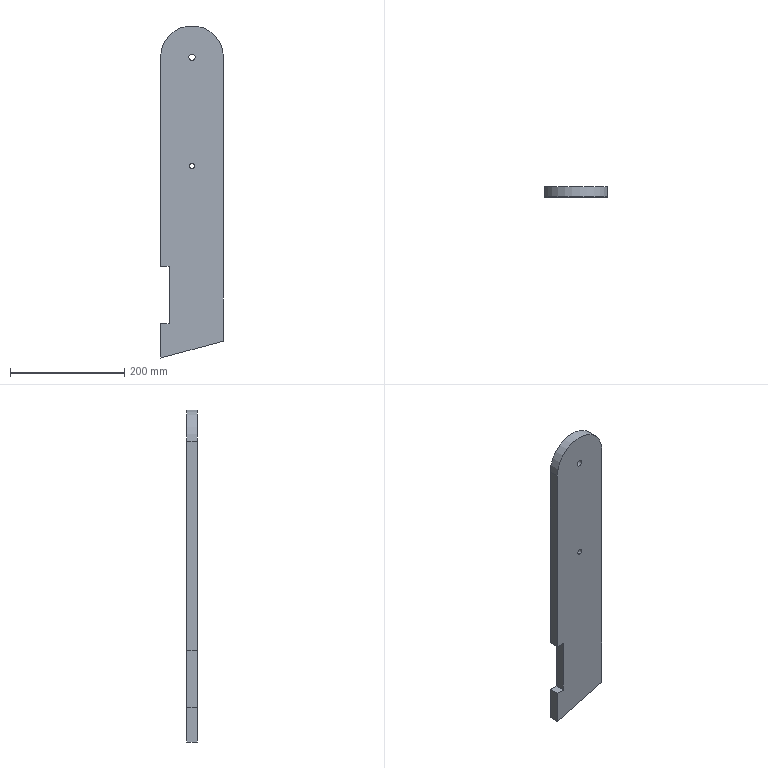Part | STEP file | Leg_left | 1 solid | 12 faces | box 110 x 18 x 580.604 mm | volume 1067190 mm3 | plane 9 | cylinder 3 | commonest cylinder face diameters 9 x1 11 x1 110 x1
STEP:
#1=CARTESIAN_POINT('',(0.,0.,0.));
#2=DIRECTION('',(0.,0.,1.));
#3=DIRECTION('',(1.,0.,0.));
#4=AXIS2_PLACEMENT_3D('',#1,#2,#3);
#5=CARTESIAN_POINT('',(55.,0.,0.));
#6=VERTEX_POINT('',#5);
#7=CARTESIAN_POINT('',(-55.,0.,0.));
#8=VERTEX_POINT('',#7);
#9=CARTESIAN_POINT('',(0.,0.,0.));
#10=DIRECTION('',(0.,-1.,0.));
#11=DIRECTION('',(1.,0.,0.));
#12=AXIS2_PLACEMENT_3D('',#9,#10,#11);
#13=CIRCLE('',#12,55.);
#14=CARTESIAN_POINT('',(0.,0.,0.));
#15=DIRECTION('',(0.,1.,0.));
#16=DIRECTION('',(1.,0.,0.));
#17=AXIS2_PLACEMENT_3D('',#14,#15,#16);
#18=CYLINDRICAL_SURFACE('',#17,55.);
#19=CARTESIAN_POINT('',(6.283,0.));
#20=DIRECTION('',(-1.,0.));
#21=VECTOR('',#20,1.);
#22=LINE('',#19,#21);
#23=(GEOMETRIC_REPRESENTATION_CONTEXT(2)PARAMETRIC_REPRESENTATION_CONTEXT()REPRESENTATION_CONTEXT('',''));
#24=DEFINITIONAL_REPRESENTATION('',(#22),#23);
#25=PCURVE('',#18,#24);
#26=CARTESIAN_POINT('',(0.7753,0.,-247.983));
#27=DIRECTION('',(0.,1.,0.));
#28=DIRECTION('',(0.,0.,1.));
#29=AXIS2_PLACEMENT_3D('',#26,#27,#28);
#30=PLANE('',#29);
#31=CARTESIAN_POINT('',(247.983,54.225));
#32=CARTESIAN_POINT('',(343.246,54.225));
#33=CARTESIAN_POINT('',(295.614,-28.275));
#34=CARTESIAN_POINT('',(247.983,-110.775));
#35=CARTESIAN_POINT('',(200.351,-28.275));
#36=CARTESIAN_POINT('',(152.72,54.225));
#37=CARTESIAN_POINT('',(247.983,54.225));
#38=(BOUNDED_CURVE()B_SPLINE_CURVE(2,(#31,#32,#33,#34,#35,#36,#37),.UNSPECIFIED.,.T.,.F.)B_SPLINE_CURVE_WITH_KNOTS((1,2,2,2,2,1),(-2.094,0.,2.094,4.189,6.283,8.378),.UNSPECIFIED.)CURVE()GEOMETRIC_REPRESENTATION_ITEM()RATIONAL_B_SPLINE_CURVE((1.,0.5,1.,0.5,1.,0.5,1.))REPRESENTATION_ITEM(''));
#39=(GEOMETRIC_REPRESENTATION_CONTEXT(2)PARAMETRIC_REPRESENTATION_CONTEXT()REPRESENTATION_CONTEXT('',''));
#40=DEFINITIONAL_REPRESENTATION('',(#38),#39);
#41=PCURVE('',#30,#40);
#42=SURFACE_CURVE('',#13,(#25,#41),.PCURVE_S1.);
#43=EDGE_CURVE('',#6,#8,#42,.T.);
#44=ORIENTED_EDGE('',*,*,#43,.T.);
#45=CARTESIAN_POINT('',(-55.,-18.,0.));
#46=VERTEX_POINT('',#45);
#47=CARTESIAN_POINT('',(-55.,0.,0.));
#48=DIRECTION('',(0.,-1.,0.));
#49=VECTOR('',#48,1.);
#50=LINE('',#47,#49);
#51=CARTESIAN_POINT('',(3.142,0.));
#52=DIRECTION('',(0.,-1.));
#53=VECTOR('',#52,1.);
#54=LINE('',#51,#53);
#55=(GEOMETRIC_REPRESENTATION_CONTEXT(2)PARAMETRIC_REPRESENTATION_CONTEXT()REPRESENTATION_CONTEXT('',''));
#56=DEFINITIONAL_REPRESENTATION('',(#54),#55);
#57=PCURVE('',#18,#56);
#58=CARTESIAN_POINT('',(-55.,0.,0.));
#59=DIRECTION('',(1.,0.,0.));
#60=DIRECTION('',(0.,0.,-1.));
#61=AXIS2_PLACEMENT_3D('',#58,#59,#60);
#62=PLANE('',#61);
#63=CARTESIAN_POINT('',(0.,0.));
#64=DIRECTION('',(0.,-1.));
#65=VECTOR('',#64,1.);
#66=LINE('',#63,#65);
#67=(GEOMETRIC_REPRESENTATION_CONTEXT(2)PARAMETRIC_REPRESENTATION_CONTEXT()REPRESENTATION_CONTEXT('',''));
#68=DEFINITIONAL_REPRESENTATION('',(#66),#67);
#69=PCURVE('',#62,#68);
#70=SURFACE_CURVE('',#50,(#57,#69),.PCURVE_S1.);
#71=EDGE_CURVE('',#8,#46,#70,.T.);
#72=ORIENTED_EDGE('',*,*,#71,.T.);
#73=CARTESIAN_POINT('',(55.,-18.,0.));
#74=VERTEX_POINT('',#73);
#75=CARTESIAN_POINT('',(0.,-18.,0.));
#76=DIRECTION('',(0.,-1.,0.));
#77=DIRECTION('',(1.,0.,0.));
#78=AXIS2_PLACEMENT_3D('',#75,#76,#77);
#79=CIRCLE('',#78,55.);
#80=CARTESIAN_POINT('',(6.283,-18.));
#81=DIRECTION('',(-1.,0.));
#82=VECTOR('',#81,1.);
#83=LINE('',#80,#82);
#84=(GEOMETRIC_REPRESENTATION_CONTEXT(2)PARAMETRIC_REPRESENTATION_CONTEXT()REPRESENTATION_CONTEXT('',''));
#85=DEFINITIONAL_REPRESENTATION('',(#83),#84);
#86=PCURVE('',#18,#85);
#87=CARTESIAN_POINT('',(0.7753,-18.,-247.983));
#88=DIRECTION('',(0.,1.,0.));
#89=DIRECTION('',(0.,0.,1.));
#90=AXIS2_PLACEMENT_3D('',#87,#88,#89);
#91=PLANE('',#90);
#92=CARTESIAN_POINT('',(247.983,54.225));
#93=CARTESIAN_POINT('',(343.246,54.225));
#94=CARTESIAN_POINT('',(295.614,-28.275));
#95=CARTESIAN_POINT('',(247.983,-110.775));
#96=CARTESIAN_POINT('',(200.351,-28.275));
#97=CARTESIAN_POINT('',(152.72,54.225));
#98=CARTESIAN_POINT('',(247.983,54.225));
#99=(BOUNDED_CURVE()B_SPLINE_CURVE(2,(#92,#93,#94,#95,#96,#97,#98),.UNSPECIFIED.,.T.,.F.)B_SPLINE_CURVE_WITH_KNOTS((1,2,2,2,2,1),(-2.094,0.,2.094,4.189,6.283,8.378),.UNSPECIFIED.)CURVE()GEOMETRIC_REPRESENTATION_ITEM()RATIONAL_B_SPLINE_CURVE((1.,0.5,1.,0.5,1.,0.5,1.))REPRESENTATION_ITEM(''));
#100=(GEOMETRIC_REPRESENTATION_CONTEXT(2)PARAMETRIC_REPRESENTATION_CONTEXT()REPRESENTATION_CONTEXT('',''));
#101=DEFINITIONAL_REPRESENTATION('',(#99),#100);
#102=PCURVE('',#91,#101);
#103=SURFACE_CURVE('',#79,(#86,#102),.PCURVE_S1.);
#104=EDGE_CURVE('',#74,#46,#103,.T.);
#105=ORIENTED_EDGE('',*,*,#104,.F.);
#106=CARTESIAN_POINT('',(55.,0.,0.));
#107=DIRECTION('',(0.,-1.,0.));
#108=VECTOR('',#107,1.);
#109=LINE('',#106,#108);
#110=CARTESIAN_POINT('',(6.283,0.));
#111=DIRECTION('',(0.,-1.));
#112=VECTOR('',#111,1.);
#113=LINE('',#110,#112);
#114=(GEOMETRIC_REPRESENTATION_CONTEXT(2)PARAMETRIC_REPRESENTATION_CONTEXT()REPRESENTATION_CONTEXT('',''));
#115=DEFINITIONAL_REPRESENTATION('',(#113),#114);
#116=PCURVE('',#18,#115);
#117=CARTESIAN_POINT('',(55.,0.,0.));
#118=DIRECTION('',(1.,0.,0.));
#119=DIRECTION('',(0.,0.,-1.));
#120=AXIS2_PLACEMENT_3D('',#117,#118,#119);
#121=PLANE('',#120);
#122=CARTESIAN_POINT('',(0.,0.));
#123=DIRECTION('',(0.,-1.));
#124=VECTOR('',#123,1.);
#125=LINE('',#122,#124);
#126=(GEOMETRIC_REPRESENTATION_CONTEXT(2)PARAMETRIC_REPRESENTATION_CONTEXT()REPRESENTATION_CONTEXT('',''));
#127=DEFINITIONAL_REPRESENTATION('',(#125),#126);
#128=PCURVE('',#121,#127);
#129=SURFACE_CURVE('',#109,(#116,#128),.PCURVE_S1.);
#130=EDGE_CURVE('',#6,#74,#129,.T.);
#131=ORIENTED_EDGE('',*,*,#130,.F.);
#132=EDGE_LOOP('',(#44,#72,#105,#131));
#133=FACE_BOUND('',#132,.T.);
#134=ADVANCED_FACE('',(#133),#18,.T.);
#135=ORIENTED_EDGE('',*,*,#130,.T.);
#136=CARTESIAN_POINT('',(55.,-18.,-496.13));
#137=VERTEX_POINT('',#136);
#138=CARTESIAN_POINT('',(55.,-18.,0.));
#139=DIRECTION('',(0.,0.,-1.));
#140=VECTOR('',#139,1.);
#141=LINE('',#138,#140);
#142=CARTESIAN_POINT('',(0.,-18.));
#143=DIRECTION('',(1.,0.));
#144=VECTOR('',#143,1.);
#145=LINE('',#142,#144);
#146=(GEOMETRIC_REPRESENTATION_CONTEXT(2)PARAMETRIC_REPRESENTATION_CONTEXT()REPRESENTATION_CONTEXT('',''));
#147=DEFINITIONAL_REPRESENTATION('',(#145),#146);
#148=PCURVE('',#121,#147);
#149=CARTESIAN_POINT('',(247.983,54.225));
#150=DIRECTION('',(-1.,0.));
#151=VECTOR('',#150,1.);
#152=LINE('',#149,#151);
#153=(GEOMETRIC_REPRESENTATION_CONTEXT(2)PARAMETRIC_REPRESENTATION_CONTEXT()REPRESENTATION_CONTEXT('',''));
#154=DEFINITIONAL_REPRESENTATION('',(#152),#153);
#155=PCURVE('',#91,#154);
#156=SURFACE_CURVE('',#141,(#148,#155),.PCURVE_S1.);
#157=EDGE_CURVE('',#74,#137,#156,.T.);
#158=ORIENTED_EDGE('',*,*,#157,.T.);
#159=CARTESIAN_POINT('',(55.,0.,-496.13));
#160=VERTEX_POINT('',#159);
#161=CARTESIAN_POINT('',(55.,0.,-496.13));
#162=DIRECTION('',(0.,-1.,0.));
#163=VECTOR('',#162,1.);
#164=LINE('',#161,#163);
#165=CARTESIAN_POINT('',(496.13,0.));
#166=DIRECTION('',(0.,-1.));
#167=VECTOR('',#166,1.);
#168=LINE('',#165,#167);
#169=(GEOMETRIC_REPRESENTATION_CONTEXT(2)PARAMETRIC_REPRESENTATION_CONTEXT()REPRESENTATION_CONTEXT('',''));
#170=DEFINITIONAL_REPRESENTATION('',(#168),#169);
#171=PCURVE('',#121,#170);
#172=CARTESIAN_POINT('',(-55.,0.,-525.604));
#173=DIRECTION('',(-0.2588,0.,0.9659));
#174=DIRECTION('',(0.9659,0.,0.2588));
#175=AXIS2_PLACEMENT_3D('',#172,#173,#174);
#176=PLANE('',#175);
#177=CARTESIAN_POINT('',(113.88,0.));
#178=DIRECTION('',(0.,-1.));
#179=VECTOR('',#178,1.);
#180=LINE('',#177,#179);
#181=(GEOMETRIC_REPRESENTATION_CONTEXT(2)PARAMETRIC_REPRESENTATION_CONTEXT()REPRESENTATION_CONTEXT('',''));
#182=DEFINITIONAL_REPRESENTATION('',(#180),#181);
#183=PCURVE('',#176,#182);
#184=SURFACE_CURVE('',#164,(#171,#183),.PCURVE_S1.);
#185=EDGE_CURVE('',#160,#137,#184,.T.);
#186=ORIENTED_EDGE('',*,*,#185,.F.);
#187=CARTESIAN_POINT('',(55.,0.,0.));
#188=DIRECTION('',(0.,0.,-1.));
#189=VECTOR('',#188,1.);
#190=LINE('',#187,#189);
#191=CARTESIAN_POINT('',(0.,0.));
#192=DIRECTION('',(1.,0.));
#193=VECTOR('',#192,1.);
#194=LINE('',#191,#193);
#195=(GEOMETRIC_REPRESENTATION_CONTEXT(2)PARAMETRIC_REPRESENTATION_CONTEXT()REPRESENTATION_CONTEXT('',''));
#196=DEFINITIONAL_REPRESENTATION('',(#194),#195);
#197=PCURVE('',#121,#196);
#198=CARTESIAN_POINT('',(247.983,54.225));
#199=DIRECTION('',(-1.,0.));
#200=VECTOR('',#199,1.);
#201=LINE('',#198,#200);
#202=(GEOMETRIC_REPRESENTATION_CONTEXT(2)PARAMETRIC_REPRESENTATION_CONTEXT()REPRESENTATION_CONTEXT('',''));
#203=DEFINITIONAL_REPRESENTATION('',(#201),#202);
#204=PCURVE('',#30,#203);
#205=SURFACE_CURVE('',#190,(#197,#204),.PCURVE_S1.);
#206=EDGE_CURVE('',#6,#160,#205,.T.);
#207=ORIENTED_EDGE('',*,*,#206,.F.);
#208=EDGE_LOOP('',(#135,#158,#186,#207));
#209=FACE_BOUND('',#208,.T.);
#210=ADVANCED_FACE('',(#209),#121,.T.);
#211=CARTESIAN_POINT('',(-55.,0.,-365.604));
#212=VERTEX_POINT('',#211);
#213=CARTESIAN_POINT('',(-55.,0.,0.));
#214=DIRECTION('',(0.,0.,-1.));
#215=VECTOR('',#214,1.);
#216=LINE('',#213,#215);
#217=CARTESIAN_POINT('',(0.,0.));
#218=DIRECTION('',(1.,0.));
#219=VECTOR('',#218,1.);
#220=LINE('',#217,#219);
#221=(GEOMETRIC_REPRESENTATION_CONTEXT(2)PARAMETRIC_REPRESENTATION_CONTEXT()REPRESENTATION_CONTEXT('',''));
#222=DEFINITIONAL_REPRESENTATION('',(#220),#221);
#223=PCURVE('',#62,#222);
#224=CARTESIAN_POINT('',(247.983,-55.775));
#225=DIRECTION('',(-1.,0.));
#226=VECTOR('',#225,1.);
#227=LINE('',#224,#226);
#228=(GEOMETRIC_REPRESENTATION_CONTEXT(2)PARAMETRIC_REPRESENTATION_CONTEXT()REPRESENTATION_CONTEXT('',''));
#229=DEFINITIONAL_REPRESENTATION('',(#227),#228);
#230=PCURVE('',#30,#229);
#231=SURFACE_CURVE('',#216,(#223,#230),.PCURVE_S1.);
#232=EDGE_CURVE('',#8,#212,#231,.T.);
#233=ORIENTED_EDGE('',*,*,#232,.F.);
#234=ORIENTED_EDGE('',*,*,#71,.T.);
#235=CARTESIAN_POINT('',(-55.,-18.,-365.604));
#236=VERTEX_POINT('',#235);
#237=CARTESIAN_POINT('',(-55.,-18.,0.));
#238=DIRECTION('',(0.,0.,-1.));
#239=VECTOR('',#238,1.);
#240=LINE('',#237,#239);
#241=CARTESIAN_POINT('',(0.,-18.));
#242=DIRECTION('',(1.,0.));
#243=VECTOR('',#242,1.);
#244=LINE('',#241,#243);
#245=(GEOMETRIC_REPRESENTATION_CONTEXT(2)PARAMETRIC_REPRESENTATION_CONTEXT()REPRESENTATION_CONTEXT('',''));
#246=DEFINITIONAL_REPRESENTATION('',(#244),#245);
#247=PCURVE('',#62,#246);
#248=CARTESIAN_POINT('',(247.983,-55.775));
#249=DIRECTION('',(-1.,0.));
#250=VECTOR('',#249,1.);
#251=LINE('',#248,#250);
#252=(GEOMETRIC_REPRESENTATION_CONTEXT(2)PARAMETRIC_REPRESENTATION_CONTEXT()REPRESENTATION_CONTEXT('',''));
#253=DEFINITIONAL_REPRESENTATION('',(#251),#252);
#254=PCURVE('',#91,#253);
#255=SURFACE_CURVE('',#240,(#247,#254),.PCURVE_S1.);
#256=EDGE_CURVE('',#46,#236,#255,.T.);
#257=ORIENTED_EDGE('',*,*,#256,.T.);
#258=CARTESIAN_POINT('',(-55.,0.,-365.604));
#259=DIRECTION('',(0.,-1.,0.));
#260=VECTOR('',#259,1.);
#261=LINE('',#258,#260);
#262=CARTESIAN_POINT('',(365.604,0.));
#263=DIRECTION('',(0.,-1.));
#264=VECTOR('',#263,1.);
#265=LINE('',#262,#264);
#266=(GEOMETRIC_REPRESENTATION_CONTEXT(2)PARAMETRIC_REPRESENTATION_CONTEXT()REPRESENTATION_CONTEXT('',''));
#267=DEFINITIONAL_REPRESENTATION('',(#265),#266);
#268=PCURVE('',#62,#267);
#269=CARTESIAN_POINT('',(-40.,0.,-365.604));
#270=DIRECTION('',(0.,0.,-1.));
#271=DIRECTION('',(-1.,0.,0.));
#272=AXIS2_PLACEMENT_3D('',#269,#270,#271);
#273=PLANE('',#272);
#274=CARTESIAN_POINT('',(15.,0.));
#275=DIRECTION('',(0.,-1.));
#276=VECTOR('',#275,1.);
#277=LINE('',#274,#276);
#278=(GEOMETRIC_REPRESENTATION_CONTEXT(2)PARAMETRIC_REPRESENTATION_CONTEXT()REPRESENTATION_CONTEXT('',''));
#279=DEFINITIONAL_REPRESENTATION('',(#277),#278);
#280=PCURVE('',#273,#279);
#281=SURFACE_CURVE('',#261,(#268,#280),.PCURVE_S1.);
#282=EDGE_CURVE('',#212,#236,#281,.T.);
#283=ORIENTED_EDGE('',*,*,#282,.F.);
#284=EDGE_LOOP('',(#233,#234,#257,#283));
#285=FACE_BOUND('',#284,.F.);
#286=ADVANCED_FACE('',(#285),#62,.F.);
#287=ORIENTED_EDGE('',*,*,#43,.F.);
#288=ORIENTED_EDGE('',*,*,#206,.T.);
#289=CARTESIAN_POINT('',(-55.,0.,-525.604));
#290=VERTEX_POINT('',#289);
#291=CARTESIAN_POINT('',(5.722,0.,-509.334));
#292=DIRECTION('',(0.9659,0.,0.2588));
#293=VECTOR('',#292,1.);
#294=LINE('',#291,#293);
#295=CARTESIAN_POINT('',(-261.351,4.947));
#296=DIRECTION('',(0.2588,0.9659));
#297=VECTOR('',#296,1.);
#298=LINE('',#295,#297);
#299=(GEOMETRIC_REPRESENTATION_CONTEXT(2)PARAMETRIC_REPRESENTATION_CONTEXT()REPRESENTATION_CONTEXT('',''));
#300=DEFINITIONAL_REPRESENTATION('',(#298),#299);
#301=PCURVE('',#30,#300);
#302=CARTESIAN_POINT('',(62.864,0.));
#303=DIRECTION('',(1.,0.));
#304=VECTOR('',#303,1.);
#305=LINE('',#302,#304);
#306=(GEOMETRIC_REPRESENTATION_CONTEXT(2)PARAMETRIC_REPRESENTATION_CONTEXT()REPRESENTATION_CONTEXT('',''));
#307=DEFINITIONAL_REPRESENTATION('',(#305),#306);
#308=PCURVE('',#176,#307);
#309=SURFACE_CURVE('',#294,(#301,#308),.PCURVE_S1.);
#310=EDGE_CURVE('',#290,#160,#309,.T.);
#311=ORIENTED_EDGE('',*,*,#310,.F.);
#312=CARTESIAN_POINT('',(-55.,0.,-465.604));
#313=VERTEX_POINT('',#312);
#314=CARTESIAN_POINT('',(-55.,0.,0.));
#315=DIRECTION('',(0.,0.,-1.));
#316=VECTOR('',#315,1.);
#317=LINE('',#314,#316);
#318=CARTESIAN_POINT('',(247.983,-55.775));
#319=DIRECTION('',(-1.,0.));
#320=VECTOR('',#319,1.);
#321=LINE('',#318,#320);
#322=(GEOMETRIC_REPRESENTATION_CONTEXT(2)PARAMETRIC_REPRESENTATION_CONTEXT()REPRESENTATION_CONTEXT('',''));
#323=DEFINITIONAL_REPRESENTATION('',(#321),#322);
#324=PCURVE('',#30,#323);
#325=CARTESIAN_POINT('',(-55.,0.,0.));
#326=DIRECTION('',(1.,0.,0.));
#327=DIRECTION('',(0.,0.,-1.));
#328=AXIS2_PLACEMENT_3D('',#325,#326,#327);
#329=PLANE('',#328);
#330=CARTESIAN_POINT('',(0.,0.));
#331=DIRECTION('',(1.,0.));
#332=VECTOR('',#331,1.);
#333=LINE('',#330,#332);
#334=(GEOMETRIC_REPRESENTATION_CONTEXT(2)PARAMETRIC_REPRESENTATION_CONTEXT()REPRESENTATION_CONTEXT('',''));
#335=DEFINITIONAL_REPRESENTATION('',(#333),#334);
#336=PCURVE('',#329,#335);
#337=SURFACE_CURVE('',#317,(#324,#336),.PCURVE_S1.);
#338=EDGE_CURVE('',#313,#290,#337,.T.);
#339=ORIENTED_EDGE('',*,*,#338,.F.);
#340=CARTESIAN_POINT('',(-40.,0.,-465.604));
#341=VERTEX_POINT('',#340);
#342=CARTESIAN_POINT('',(-55.,0.,-465.604));
#343=DIRECTION('',(1.,0.,0.));
#344=VECTOR('',#343,1.);
#345=LINE('',#342,#344);
#346=CARTESIAN_POINT('',(-217.621,-55.775));
#347=DIRECTION('',(0.,1.));
#348=VECTOR('',#347,1.);
#349=LINE('',#346,#348);
#350=(GEOMETRIC_REPRESENTATION_CONTEXT(2)PARAMETRIC_REPRESENTATION_CONTEXT()REPRESENTATION_CONTEXT('',''));
#351=DEFINITIONAL_REPRESENTATION('',(#349),#350);
#352=PCURVE('',#30,#351);
#353=CARTESIAN_POINT('',(-55.,0.,-465.604));
#354=DIRECTION('',(0.,0.,1.));
#355=DIRECTION('',(1.,0.,0.));
#356=AXIS2_PLACEMENT_3D('',#353,#354,#355);
#357=PLANE('',#356);
#358=CARTESIAN_POINT('',(0.,0.));
#359=DIRECTION('',(1.,0.));
#360=VECTOR('',#359,1.);
#361=LINE('',#358,#360);
#362=(GEOMETRIC_REPRESENTATION_CONTEXT(2)PARAMETRIC_REPRESENTATION_CONTEXT()REPRESENTATION_CONTEXT('',''));
#363=DEFINITIONAL_REPRESENTATION('',(#361),#362);
#364=PCURVE('',#357,#363);
#365=SURFACE_CURVE('',#345,(#352,#364),.PCURVE_S1.);
#366=EDGE_CURVE('',#313,#341,#365,.T.);
#367=ORIENTED_EDGE('',*,*,#366,.T.);
#368=CARTESIAN_POINT('',(-40.,0.,-365.604));
#369=VERTEX_POINT('',#368);
#370=CARTESIAN_POINT('',(-40.,0.,-465.604));
#371=DIRECTION('',(0.,0.,1.));
#372=VECTOR('',#371,1.);
#373=LINE('',#370,#372);
#374=CARTESIAN_POINT('',(-217.621,-40.775));
#375=DIRECTION('',(1.,0.));
#376=VECTOR('',#375,1.);
#377=LINE('',#374,#376);
#378=(GEOMETRIC_REPRESENTATION_CONTEXT(2)PARAMETRIC_REPRESENTATION_CONTEXT()REPRESENTATION_CONTEXT('',''));
#379=DEFINITIONAL_REPRESENTATION('',(#377),#378);
#380=PCURVE('',#30,#379);
#381=CARTESIAN_POINT('',(-40.,0.,-465.604));
#382=DIRECTION('',(-1.,0.,0.));
#383=DIRECTION('',(0.,0.,1.));
#384=AXIS2_PLACEMENT_3D('',#381,#382,#383);
#385=PLANE('',#384);
#386=CARTESIAN_POINT('',(0.,0.));
#387=DIRECTION('',(1.,0.));
#388=VECTOR('',#387,1.);
#389=LINE('',#386,#388);
#390=(GEOMETRIC_REPRESENTATION_CONTEXT(2)PARAMETRIC_REPRESENTATION_CONTEXT()REPRESENTATION_CONTEXT('',''));
#391=DEFINITIONAL_REPRESENTATION('',(#389),#390);
#392=PCURVE('',#385,#391);
#393=SURFACE_CURVE('',#373,(#380,#392),.PCURVE_S1.);
#394=EDGE_CURVE('',#341,#369,#393,.T.);
#395=ORIENTED_EDGE('',*,*,#394,.T.);
#396=CARTESIAN_POINT('',(-40.,0.,-365.604));
#397=DIRECTION('',(-1.,0.,0.));
#398=VECTOR('',#397,1.);
#399=LINE('',#396,#398);
#400=CARTESIAN_POINT('',(-117.621,-40.775));
#401=DIRECTION('',(0.,-1.));
#402=VECTOR('',#401,1.);
#403=LINE('',#400,#402);
#404=(GEOMETRIC_REPRESENTATION_CONTEXT(2)PARAMETRIC_REPRESENTATION_CONTEXT()REPRESENTATION_CONTEXT('',''));
#405=DEFINITIONAL_REPRESENTATION('',(#403),#404);
#406=PCURVE('',#30,#405);
#407=CARTESIAN_POINT('',(0.,0.));
#408=DIRECTION('',(1.,0.));
#409=VECTOR('',#408,1.);
#410=LINE('',#407,#409);
#411=(GEOMETRIC_REPRESENTATION_CONTEXT(2)PARAMETRIC_REPRESENTATION_CONTEXT()REPRESENTATION_CONTEXT('',''));
#412=DEFINITIONAL_REPRESENTATION('',(#410),#411);
#413=PCURVE('',#273,#412);
#414=SURFACE_CURVE('',#399,(#406,#413),.PCURVE_S1.);
#415=EDGE_CURVE('',#369,#212,#414,.T.);
#416=ORIENTED_EDGE('',*,*,#415,.T.);
#417=ORIENTED_EDGE('',*,*,#232,.F.);
#418=EDGE_LOOP('',(#287,#288,#311,#339,#367,#395,#416,#417));
#419=FACE_BOUND('',#418,.T.);
#420=CARTESIAN_POINT('',(-4.5,0.,-190.));
#421=VERTEX_POINT('',#420);
#422=CARTESIAN_POINT('',(0.,0.,-190.));
#423=DIRECTION('',(0.,1.,0.));
#424=DIRECTION('',(-1.,0.,0.));
#425=AXIS2_PLACEMENT_3D('',#422,#423,#424);
#426=CIRCLE('',#425,4.5);
#427=CARTESIAN_POINT('',(57.983,-0.7753));
#428=DIRECTION('',(0.,-1.));
#429=AXIS2_PLACEMENT_2D('',#427,#428);
#430=CIRCLE('',#429,4.5);
#431=(GEOMETRIC_REPRESENTATION_CONTEXT(2)PARAMETRIC_REPRESENTATION_CONTEXT()REPRESENTATION_CONTEXT('',''));
#432=DEFINITIONAL_REPRESENTATION('',(#430),#431);
#433=PCURVE('',#30,#432);
#434=CARTESIAN_POINT('',(0.,-18.,-190.));
#435=DIRECTION('',(0.,1.,0.));
#436=DIRECTION('',(-1.,0.,0.));
#437=AXIS2_PLACEMENT_3D('',#434,#435,#436);
#438=CYLINDRICAL_SURFACE('',#437,4.5);
#439=CARTESIAN_POINT('',(0.,18.));
#440=DIRECTION('',(1.,0.));
#441=VECTOR('',#440,1.);
#442=LINE('',#439,#441);
#443=(GEOMETRIC_REPRESENTATION_CONTEXT(2)PARAMETRIC_REPRESENTATION_CONTEXT()REPRESENTATION_CONTEXT('',''));
#444=DEFINITIONAL_REPRESENTATION('',(#442),#443);
#445=PCURVE('',#438,#444);
#446=SURFACE_CURVE('',#426,(#433,#445),.PCURVE_S1.);
#447=EDGE_CURVE('',#421,#421,#446,.T.);
#448=ORIENTED_EDGE('',*,*,#447,.F.);
#449=EDGE_LOOP('',(#448));
#450=FACE_BOUND('',#449,.T.);
#451=CARTESIAN_POINT('',(5.5,0.,0.));
#452=VERTEX_POINT('',#451);
#453=CARTESIAN_POINT('',(0.,0.,0.));
#454=DIRECTION('',(0.,-1.,0.));
#455=DIRECTION('',(1.,0.,0.));
#456=AXIS2_PLACEMENT_3D('',#453,#454,#455);
#457=CIRCLE('',#456,5.5);
#458=CARTESIAN_POINT('',(247.983,4.725));
#459=CARTESIAN_POINT('',(257.509,4.725));
#460=CARTESIAN_POINT('',(252.746,-3.525));
#461=CARTESIAN_POINT('',(247.983,-11.775));
#462=CARTESIAN_POINT('',(243.22,-3.525));
#463=CARTESIAN_POINT('',(238.456,4.725));
#464=CARTESIAN_POINT('',(247.983,4.725));
#465=(BOUNDED_CURVE()B_SPLINE_CURVE(2,(#458,#459,#460,#461,#462,#463,#464),.UNSPECIFIED.,.T.,.F.)B_SPLINE_CURVE_WITH_KNOTS((1,2,2,2,2,1),(-2.094,0.,2.094,4.189,6.283,8.378),.UNSPECIFIED.)CURVE()GEOMETRIC_REPRESENTATION_ITEM()RATIONAL_B_SPLINE_CURVE((1.,0.5,1.,0.5,1.,0.5,1.))REPRESENTATION_ITEM(''));
#466=(GEOMETRIC_REPRESENTATION_CONTEXT(2)PARAMETRIC_REPRESENTATION_CONTEXT()REPRESENTATION_CONTEXT('',''));
#467=DEFINITIONAL_REPRESENTATION('',(#465),#466);
#468=PCURVE('',#30,#467);
#469=CARTESIAN_POINT('',(0.,0.,0.));
#470=DIRECTION('',(0.,1.,0.));
#471=DIRECTION('',(1.,0.,0.));
#472=AXIS2_PLACEMENT_3D('',#469,#470,#471);
#473=CYLINDRICAL_SURFACE('',#472,5.5);
#474=CARTESIAN_POINT('',(6.283,0.));
#475=DIRECTION('',(-1.,0.));
#476=VECTOR('',#475,1.);
#477=LINE('',#474,#476);
#478=(GEOMETRIC_REPRESENTATION_CONTEXT(2)PARAMETRIC_REPRESENTATION_CONTEXT()REPRESENTATION_CONTEXT('',''));
#479=DEFINITIONAL_REPRESENTATION('',(#477),#478);
#480=PCURVE('',#473,#479);
#481=SURFACE_CURVE('',#457,(#468,#480),.PCURVE_S1.);
#482=EDGE_CURVE('',#452,#452,#481,.T.);
#483=ORIENTED_EDGE('',*,*,#482,.T.);
#484=EDGE_LOOP('',(#483));
#485=FACE_BOUND('',#484,.T.);
#486=ADVANCED_FACE('',(#419,#450,#485),#30,.T.);
#487=ORIENTED_EDGE('',*,*,#104,.F.);
#488=ORIENTED_EDGE('',*,*,#157,.T.);
#489=CARTESIAN_POINT('',(-55.,-18.,-525.604));
#490=VERTEX_POINT('',#489);
#491=CARTESIAN_POINT('',(5.722,-18.,-509.334));
#492=DIRECTION('',(0.9659,0.,0.2588));
#493=VECTOR('',#492,1.);
#494=LINE('',#491,#493);
#495=CARTESIAN_POINT('',(-261.351,4.947));
#496=DIRECTION('',(0.2588,0.9659));
#497=VECTOR('',#496,1.);
#498=LINE('',#495,#497);
#499=(GEOMETRIC_REPRESENTATION_CONTEXT(2)PARAMETRIC_REPRESENTATION_CONTEXT()REPRESENTATION_CONTEXT('',''));
#500=DEFINITIONAL_REPRESENTATION('',(#498),#499);
#501=PCURVE('',#91,#500);
#502=CARTESIAN_POINT('',(62.864,-18.));
#503=DIRECTION('',(1.,0.));
#504=VECTOR('',#503,1.);
#505=LINE('',#502,#504);
#506=(GEOMETRIC_REPRESENTATION_CONTEXT(2)PARAMETRIC_REPRESENTATION_CONTEXT()REPRESENTATION_CONTEXT('',''));
#507=DEFINITIONAL_REPRESENTATION('',(#505),#506);
#508=PCURVE('',#176,#507);
#509=SURFACE_CURVE('',#494,(#501,#508),.PCURVE_S1.);
#510=EDGE_CURVE('',#490,#137,#509,.T.);
#511=ORIENTED_EDGE('',*,*,#510,.F.);
#512=CARTESIAN_POINT('',(-55.,-18.,-465.604));
#513=VERTEX_POINT('',#512);
#514=CARTESIAN_POINT('',(-55.,-18.,0.));
#515=DIRECTION('',(0.,0.,-1.));
#516=VECTOR('',#515,1.);
#517=LINE('',#514,#516);
#518=CARTESIAN_POINT('',(247.983,-55.775));
#519=DIRECTION('',(-1.,0.));
#520=VECTOR('',#519,1.);
#521=LINE('',#518,#520);
#522=(GEOMETRIC_REPRESENTATION_CONTEXT(2)PARAMETRIC_REPRESENTATION_CONTEXT()REPRESENTATION_CONTEXT('',''));
#523=DEFINITIONAL_REPRESENTATION('',(#521),#522);
#524=PCURVE('',#91,#523);
#525=CARTESIAN_POINT('',(0.,-18.));
#526=DIRECTION('',(1.,0.));
#527=VECTOR('',#526,1.);
#528=LINE('',#525,#527);
#529=(GEOMETRIC_REPRESENTATION_CONTEXT(2)PARAMETRIC_REPRESENTATION_CONTEXT()REPRESENTATION_CONTEXT('',''));
#530=DEFINITIONAL_REPRESENTATION('',(#528),#529);
#531=PCURVE('',#329,#530);
#532=SURFACE_CURVE('',#517,(#524,#531),.PCURVE_S1.);
#533=EDGE_CURVE('',#513,#490,#532,.T.);
#534=ORIENTED_EDGE('',*,*,#533,.F.);
#535=CARTESIAN_POINT('',(-40.,-18.,-465.604));
#536=VERTEX_POINT('',#535);
#537=CARTESIAN_POINT('',(-27.112,-18.,-465.604));
#538=DIRECTION('',(1.,0.,0.));
#539=VECTOR('',#538,1.);
#540=LINE('',#537,#539);
#541=CARTESIAN_POINT('',(-217.621,-27.888));
#542=DIRECTION('',(0.,1.));
#543=VECTOR('',#542,1.);
#544=LINE('',#541,#543);
#545=(GEOMETRIC_REPRESENTATION_CONTEXT(2)PARAMETRIC_REPRESENTATION_CONTEXT()REPRESENTATION_CONTEXT('',''));
#546=DEFINITIONAL_REPRESENTATION('',(#544),#545);
#547=PCURVE('',#91,#546);
#548=CARTESIAN_POINT('',(27.888,-18.));
#549=DIRECTION('',(1.,0.));
#550=VECTOR('',#549,1.);
#551=LINE('',#548,#550);
#552=(GEOMETRIC_REPRESENTATION_CONTEXT(2)PARAMETRIC_REPRESENTATION_CONTEXT()REPRESENTATION_CONTEXT('',''));
#553=DEFINITIONAL_REPRESENTATION('',(#551),#552);
#554=PCURVE('',#357,#553);
#555=SURFACE_CURVE('',#540,(#547,#554),.PCURVE_S1.);
#556=EDGE_CURVE('',#513,#536,#555,.T.);
#557=ORIENTED_EDGE('',*,*,#556,.T.);
#558=CARTESIAN_POINT('',(-40.,-18.,-365.604));
#559=VERTEX_POINT('',#558);
#560=CARTESIAN_POINT('',(-40.,-18.,-356.793));
#561=DIRECTION('',(0.,0.,1.));
#562=VECTOR('',#561,1.);
#563=LINE('',#560,#562);
#564=CARTESIAN_POINT('',(-108.811,-40.775));
#565=DIRECTION('',(1.,0.));
#566=VECTOR('',#565,1.);
#567=LINE('',#564,#566);
#568=(GEOMETRIC_REPRESENTATION_CONTEXT(2)PARAMETRIC_REPRESENTATION_CONTEXT()REPRESENTATION_CONTEXT('',''));
#569=DEFINITIONAL_REPRESENTATION('',(#567),#568);
#570=PCURVE('',#91,#569);
#571=CARTESIAN_POINT('',(108.811,-18.));
#572=DIRECTION('',(1.,0.));
#573=VECTOR('',#572,1.);
#574=LINE('',#571,#573);
#575=(GEOMETRIC_REPRESENTATION_CONTEXT(2)PARAMETRIC_REPRESENTATION_CONTEXT()REPRESENTATION_CONTEXT('',''));
#576=DEFINITIONAL_REPRESENTATION('',(#574),#575);
#577=PCURVE('',#385,#576);
#578=SURFACE_CURVE('',#563,(#570,#577),.PCURVE_S1.);
#579=EDGE_CURVE('',#536,#559,#578,.T.);
#580=ORIENTED_EDGE('',*,*,#579,.T.);
#581=CARTESIAN_POINT('',(-19.612,-18.,-365.604));
#582=DIRECTION('',(-1.,0.,0.));
#583=VECTOR('',#582,1.);
#584=LINE('',#581,#583);
#585=CARTESIAN_POINT('',(-117.621,-20.388));
#586=DIRECTION('',(0.,-1.));
#587=VECTOR('',#586,1.);
#588=LINE('',#585,#587);
#589=(GEOMETRIC_REPRESENTATION_CONTEXT(2)PARAMETRIC_REPRESENTATION_CONTEXT()REPRESENTATION_CONTEXT('',''));
#590=DEFINITIONAL_REPRESENTATION('',(#588),#589);
#591=PCURVE('',#91,#590);
#592=CARTESIAN_POINT('',(-20.388,-18.));
#593=DIRECTION('',(1.,0.));
#594=VECTOR('',#593,1.);
#595=LINE('',#592,#594);
#596=(GEOMETRIC_REPRESENTATION_CONTEXT(2)PARAMETRIC_REPRESENTATION_CONTEXT()REPRESENTATION_CONTEXT('',''));
#597=DEFINITIONAL_REPRESENTATION('',(#595),#596);
#598=PCURVE('',#273,#597);
#599=SURFACE_CURVE('',#584,(#591,#598),.PCURVE_S1.);
#600=EDGE_CURVE('',#559,#236,#599,.T.);
#601=ORIENTED_EDGE('',*,*,#600,.T.);
#602=ORIENTED_EDGE('',*,*,#256,.F.);
#603=EDGE_LOOP('',(#487,#488,#511,#534,#557,#580,#601,#602));
#604=FACE_BOUND('',#603,.F.);
#605=CARTESIAN_POINT('',(-4.5,-18.,-190.));
#606=VERTEX_POINT('',#605);
#607=CARTESIAN_POINT('',(0.,-18.,-190.));
#608=DIRECTION('',(0.,-1.,0.));
#609=DIRECTION('',(-1.,0.,0.));
#610=AXIS2_PLACEMENT_3D('',#607,#608,#609);
#611=CIRCLE('',#610,4.5);
#612=CARTESIAN_POINT('',(57.983,-5.275));
#613=CARTESIAN_POINT('',(50.189,-5.275));
#614=CARTESIAN_POINT('',(54.086,1.475));
#615=CARTESIAN_POINT('',(57.983,8.225));
#616=CARTESIAN_POINT('',(61.88,1.475));
#617=CARTESIAN_POINT('',(65.777,-5.275));
#618=CARTESIAN_POINT('',(57.983,-5.275));
#619=(BOUNDED_CURVE()B_SPLINE_CURVE(2,(#612,#613,#614,#615,#616,#617,#618),.UNSPECIFIED.,.T.,.F.)B_SPLINE_CURVE_WITH_KNOTS((1,2,2,2,2,1),(-2.094,0.,2.094,4.189,6.283,8.378),.UNSPECIFIED.)CURVE()GEOMETRIC_REPRESENTATION_ITEM()RATIONAL_B_SPLINE_CURVE((1.,0.5,1.,0.5,1.,0.5,1.))REPRESENTATION_ITEM(''));
#620=(GEOMETRIC_REPRESENTATION_CONTEXT(2)PARAMETRIC_REPRESENTATION_CONTEXT()REPRESENTATION_CONTEXT('',''));
#621=DEFINITIONAL_REPRESENTATION('',(#619),#620);
#622=PCURVE('',#91,#621);
#623=CARTESIAN_POINT('',(6.283,0.));
#624=DIRECTION('',(-1.,0.));
#625=VECTOR('',#624,1.);
#626=LINE('',#623,#625);
#627=(GEOMETRIC_REPRESENTATION_CONTEXT(2)PARAMETRIC_REPRESENTATION_CONTEXT()REPRESENTATION_CONTEXT('',''));
#628=DEFINITIONAL_REPRESENTATION('',(#626),#627);
#629=PCURVE('',#438,#628);
#630=SURFACE_CURVE('',#611,(#622,#629),.PCURVE_S1.);
#631=EDGE_CURVE('',#606,#606,#630,.T.);
#632=ORIENTED_EDGE('',*,*,#631,.T.);
#633=EDGE_LOOP('',(#632));
#634=FACE_BOUND('',#633,.F.);
#635=CARTESIAN_POINT('',(5.5,-18.,0.));
#636=VERTEX_POINT('',#635);
#637=CARTESIAN_POINT('',(0.,-18.,0.));
#638=DIRECTION('',(0.,-1.,0.));
#639=DIRECTION('',(1.,0.,0.));
#640=AXIS2_PLACEMENT_3D('',#637,#638,#639);
#641=CIRCLE('',#640,5.5);
#642=CARTESIAN_POINT('',(247.983,4.725));
#643=CARTESIAN_POINT('',(257.509,4.725));
#644=CARTESIAN_POINT('',(252.746,-3.525));
#645=CARTESIAN_POINT('',(247.983,-11.775));
#646=CARTESIAN_POINT('',(243.22,-3.525));
#647=CARTESIAN_POINT('',(238.456,4.725));
#648=CARTESIAN_POINT('',(247.983,4.725));
#649=(BOUNDED_CURVE()B_SPLINE_CURVE(2,(#642,#643,#644,#645,#646,#647,#648),.UNSPECIFIED.,.T.,.F.)B_SPLINE_CURVE_WITH_KNOTS((1,2,2,2,2,1),(-2.094,0.,2.094,4.189,6.283,8.378),.UNSPECIFIED.)CURVE()GEOMETRIC_REPRESENTATION_ITEM()RATIONAL_B_SPLINE_CURVE((1.,0.5,1.,0.5,1.,0.5,1.))REPRESENTATION_ITEM(''));
#650=(GEOMETRIC_REPRESENTATION_CONTEXT(2)PARAMETRIC_REPRESENTATION_CONTEXT()REPRESENTATION_CONTEXT('',''));
#651=DEFINITIONAL_REPRESENTATION('',(#649),#650);
#652=PCURVE('',#91,#651);
#653=CARTESIAN_POINT('',(6.283,-18.));
#654=DIRECTION('',(-1.,0.));
#655=VECTOR('',#654,1.);
#656=LINE('',#653,#655);
#657=(GEOMETRIC_REPRESENTATION_CONTEXT(2)PARAMETRIC_REPRESENTATION_CONTEXT()REPRESENTATION_CONTEXT('',''));
#658=DEFINITIONAL_REPRESENTATION('',(#656),#657);
#659=PCURVE('',#473,#658);
#660=SURFACE_CURVE('',#641,(#652,#659),.PCURVE_S1.);
#661=EDGE_CURVE('',#636,#636,#660,.T.);
#662=ORIENTED_EDGE('',*,*,#661,.T.);
#663=EDGE_LOOP('',(#662));
#664=FACE_BOUND('',#663,.F.);
#665=ADVANCED_FACE('',(#604,#634,#664),#91,.F.);
#666=CARTESIAN_POINT('',(-55.,0.,-525.604));
#667=DIRECTION('',(0.,-1.,0.));
#668=VECTOR('',#667,1.);
#669=LINE('',#666,#668);
#670=CARTESIAN_POINT('',(0.,0.));
#671=DIRECTION('',(0.,-1.));
#672=VECTOR('',#671,1.);
#673=LINE('',#670,#672);
#674=(GEOMETRIC_REPRESENTATION_CONTEXT(2)PARAMETRIC_REPRESENTATION_CONTEXT()REPRESENTATION_CONTEXT('',''));
#675=DEFINITIONAL_REPRESENTATION('',(#673),#674);
#676=PCURVE('',#176,#675);
#677=CARTESIAN_POINT('',(525.604,0.));
#678=DIRECTION('',(0.,-1.));
#679=VECTOR('',#678,1.);
#680=LINE('',#677,#679);
#681=(GEOMETRIC_REPRESENTATION_CONTEXT(2)PARAMETRIC_REPRESENTATION_CONTEXT()REPRESENTATION_CONTEXT('',''));
#682=DEFINITIONAL_REPRESENTATION('',(#680),#681);
#683=PCURVE('',#329,#682);
#684=SURFACE_CURVE('',#669,(#676,#683),.PCURVE_S1.);
#685=EDGE_CURVE('',#290,#490,#684,.T.);
#686=ORIENTED_EDGE('',*,*,#685,.T.);
#687=ORIENTED_EDGE('',*,*,#510,.T.);
#688=ORIENTED_EDGE('',*,*,#185,.F.);
#689=ORIENTED_EDGE('',*,*,#310,.F.);
#690=EDGE_LOOP('',(#686,#687,#688,#689));
#691=FACE_BOUND('',#690,.F.);
#692=ADVANCED_FACE('',(#691),#176,.F.);
#693=ORIENTED_EDGE('',*,*,#415,.F.);
#694=CARTESIAN_POINT('',(-40.,0.,-365.604));
#695=DIRECTION('',(0.,-1.,0.));
#696=VECTOR('',#695,1.);
#697=LINE('',#694,#696);
#698=CARTESIAN_POINT('',(0.,0.));
#699=DIRECTION('',(0.,-1.));
#700=VECTOR('',#699,1.);
#701=LINE('',#698,#700);
#702=(GEOMETRIC_REPRESENTATION_CONTEXT(2)PARAMETRIC_REPRESENTATION_CONTEXT()REPRESENTATION_CONTEXT('',''));
#703=DEFINITIONAL_REPRESENTATION('',(#701),#702);
#704=PCURVE('',#273,#703);
#705=CARTESIAN_POINT('',(100.,0.));
#706=DIRECTION('',(0.,-1.));
#707=VECTOR('',#706,1.);
#708=LINE('',#705,#707);
#709=(GEOMETRIC_REPRESENTATION_CONTEXT(2)PARAMETRIC_REPRESENTATION_CONTEXT()REPRESENTATION_CONTEXT('',''));
#710=DEFINITIONAL_REPRESENTATION('',(#708),#709);
#711=PCURVE('',#385,#710);
#712=SURFACE_CURVE('',#697,(#704,#711),.PCURVE_S1.);
#713=EDGE_CURVE('',#369,#559,#712,.T.);
#714=ORIENTED_EDGE('',*,*,#713,.T.);
#715=ORIENTED_EDGE('',*,*,#600,.T.);
#716=ORIENTED_EDGE('',*,*,#282,.F.);
#717=EDGE_LOOP('',(#693,#714,#715,#716));
#718=FACE_BOUND('',#717,.T.);
#719=ADVANCED_FACE('',(#718),#273,.T.);
#720=ORIENTED_EDGE('',*,*,#338,.F.);
#721=CARTESIAN_POINT('',(-55.,0.,-465.604));
#722=DIRECTION('',(0.,-1.,0.));
#723=VECTOR('',#722,1.);
#724=LINE('',#721,#723);
#725=CARTESIAN_POINT('',(465.604,0.));
#726=DIRECTION('',(0.,-1.));
#727=VECTOR('',#726,1.);
#728=LINE('',#725,#727);
#729=(GEOMETRIC_REPRESENTATION_CONTEXT(2)PARAMETRIC_REPRESENTATION_CONTEXT()REPRESENTATION_CONTEXT('',''));
#730=DEFINITIONAL_REPRESENTATION('',(#728),#729);
#731=PCURVE('',#329,#730);
#732=CARTESIAN_POINT('',(0.,0.));
#733=DIRECTION('',(0.,-1.));
#734=VECTOR('',#733,1.);
#735=LINE('',#732,#734);
#736=(GEOMETRIC_REPRESENTATION_CONTEXT(2)PARAMETRIC_REPRESENTATION_CONTEXT()REPRESENTATION_CONTEXT('',''));
#737=DEFINITIONAL_REPRESENTATION('',(#735),#736);
#738=PCURVE('',#357,#737);
#739=SURFACE_CURVE('',#724,(#731,#738),.PCURVE_S1.);
#740=EDGE_CURVE('',#313,#513,#739,.T.);
#741=ORIENTED_EDGE('',*,*,#740,.T.);
#742=ORIENTED_EDGE('',*,*,#533,.T.);
#743=ORIENTED_EDGE('',*,*,#685,.F.);
#744=EDGE_LOOP('',(#720,#741,#742,#743));
#745=FACE_BOUND('',#744,.F.);
#746=ADVANCED_FACE('',(#745),#329,.F.);
#747=ORIENTED_EDGE('',*,*,#394,.F.);
#748=CARTESIAN_POINT('',(-40.,0.,-465.604));
#749=DIRECTION('',(0.,-1.,0.));
#750=VECTOR('',#749,1.);
#751=LINE('',#748,#750);
#752=CARTESIAN_POINT('',(0.,0.));
#753=DIRECTION('',(0.,-1.));
#754=VECTOR('',#753,1.);
#755=LINE('',#752,#754);
#756=(GEOMETRIC_REPRESENTATION_CONTEXT(2)PARAMETRIC_REPRESENTATION_CONTEXT()REPRESENTATION_CONTEXT('',''));
#757=DEFINITIONAL_REPRESENTATION('',(#755),#756);
#758=PCURVE('',#385,#757);
#759=CARTESIAN_POINT('',(15.,0.));
#760=DIRECTION('',(0.,-1.));
#761=VECTOR('',#760,1.);
#762=LINE('',#759,#761);
#763=(GEOMETRIC_REPRESENTATION_CONTEXT(2)PARAMETRIC_REPRESENTATION_CONTEXT()REPRESENTATION_CONTEXT('',''));
#764=DEFINITIONAL_REPRESENTATION('',(#762),#763);
#765=PCURVE('',#357,#764);
#766=SURFACE_CURVE('',#751,(#758,#765),.PCURVE_S1.);
#767=EDGE_CURVE('',#341,#536,#766,.T.);
#768=ORIENTED_EDGE('',*,*,#767,.T.);
#769=ORIENTED_EDGE('',*,*,#579,.T.);
#770=ORIENTED_EDGE('',*,*,#713,.F.);
#771=EDGE_LOOP('',(#747,#768,#769,#770));
#772=FACE_BOUND('',#771,.T.);
#773=ADVANCED_FACE('',(#772),#385,.T.);
#774=ORIENTED_EDGE('',*,*,#366,.F.);
#775=ORIENTED_EDGE('',*,*,#740,.T.);
#776=ORIENTED_EDGE('',*,*,#556,.T.);
#777=ORIENTED_EDGE('',*,*,#767,.F.);
#778=EDGE_LOOP('',(#774,#775,#776,#777));
#779=FACE_BOUND('',#778,.T.);
#780=ADVANCED_FACE('',(#779),#357,.T.);
#781=ORIENTED_EDGE('',*,*,#447,.F.);
#782=CARTESIAN_POINT('',(-4.5,-18.,-190.));
#783=DIRECTION('',(0.,1.,0.));
#784=VECTOR('',#783,1.);
#785=LINE('',#782,#784);
#786=CARTESIAN_POINT('',(0.,0.));
#787=DIRECTION('',(0.,1.));
#788=VECTOR('',#787,1.);
#789=LINE('',#786,#788);
#790=(GEOMETRIC_REPRESENTATION_CONTEXT(2)PARAMETRIC_REPRESENTATION_CONTEXT()REPRESENTATION_CONTEXT('',''));
#791=DEFINITIONAL_REPRESENTATION('',(#789),#790);
#792=PCURVE('',#438,#791);
#793=CARTESIAN_POINT('',(6.283,0.));
#794=DIRECTION('',(0.,1.));
#795=VECTOR('',#794,1.);
#796=LINE('',#793,#795);
#797=(GEOMETRIC_REPRESENTATION_CONTEXT(2)PARAMETRIC_REPRESENTATION_CONTEXT()REPRESENTATION_CONTEXT('',''));
#798=DEFINITIONAL_REPRESENTATION('',(#796),#797);
#799=PCURVE('',#438,#798);
#800=SEAM_CURVE('',#785,(#792,#799),.PCURVE_S1.);
#801=EDGE_CURVE('',#606,#421,#800,.T.);
#802=ORIENTED_EDGE('',*,*,#801,.F.);
#803=ORIENTED_EDGE('',*,*,#631,.F.);
#804=ORIENTED_EDGE('',*,*,#801,.T.);
#805=EDGE_LOOP('',(#781,#802,#803,#804));
#806=FACE_BOUND('',#805,.F.);
#807=ADVANCED_FACE('',(#806),#438,.F.);
#808=ORIENTED_EDGE('',*,*,#482,.T.);
#809=CARTESIAN_POINT('',(5.5,0.,0.));
#810=DIRECTION('',(0.,-1.,0.));
#811=VECTOR('',#810,1.);
#812=LINE('',#809,#811);
#813=CARTESIAN_POINT('',(0.,0.));
#814=DIRECTION('',(0.,-1.));
#815=VECTOR('',#814,1.);
#816=LINE('',#813,#815);
#817=(GEOMETRIC_REPRESENTATION_CONTEXT(2)PARAMETRIC_REPRESENTATION_CONTEXT()REPRESENTATION_CONTEXT('',''));
#818=DEFINITIONAL_REPRESENTATION('',(#816),#817);
#819=PCURVE('',#473,#818);
#820=CARTESIAN_POINT('',(6.283,0.));
#821=DIRECTION('',(0.,-1.));
#822=VECTOR('',#821,1.);
#823=LINE('',#820,#822);
#824=(GEOMETRIC_REPRESENTATION_CONTEXT(2)PARAMETRIC_REPRESENTATION_CONTEXT()REPRESENTATION_CONTEXT('',''));
#825=DEFINITIONAL_REPRESENTATION('',(#823),#824);
#826=PCURVE('',#473,#825);
#827=SEAM_CURVE('',#812,(#819,#826),.PCURVE_S1.);
#828=EDGE_CURVE('',#452,#636,#827,.T.);
#829=ORIENTED_EDGE('',*,*,#828,.T.);
#830=ORIENTED_EDGE('',*,*,#661,.F.);
#831=ORIENTED_EDGE('',*,*,#828,.F.);
#832=EDGE_LOOP('',(#808,#829,#830,#831));
#833=FACE_BOUND('',#832,.F.);
#834=ADVANCED_FACE('',(#833),#473,.F.);
#835=CLOSED_SHELL('',(#134,#210,#286,#486,#665,#692,#719,#746,#773,#780,#807,#834));
#836=MANIFOLD_SOLID_BREP('',#835);
#837=(LENGTH_UNIT()NAMED_UNIT(*)SI_UNIT(.MILLI.,.METRE.));
#838=UNCERTAINTY_MEASURE_WITH_UNIT(LENGTH_MEASURE(0.0000001),#837,'','');
#839=(NAMED_UNIT(*)PLANE_ANGLE_UNIT()SI_UNIT($,.RADIAN.));
#840=(NAMED_UNIT(*)SI_UNIT($,.STERADIAN.)SOLID_ANGLE_UNIT());
#841=(GEOMETRIC_REPRESENTATION_CONTEXT(3)GLOBAL_UNCERTAINTY_ASSIGNED_CONTEXT((#838))GLOBAL_UNIT_ASSIGNED_CONTEXT((#837,#839,#840))REPRESENTATION_CONTEXT('',''));
#842=ADVANCED_BREP_SHAPE_REPRESENTATION('',(#4,#836),#841);